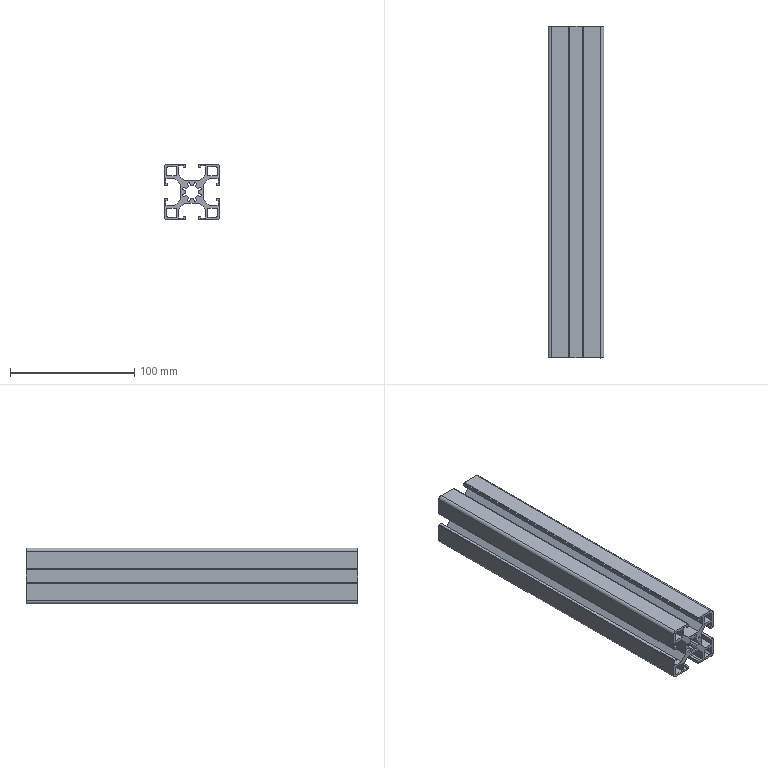Part | STEP file | 1 solid | 135 faces | box 45 x 267.5 x 45 mm | volume 185188 mm3 | plane 118 | cylinder 17 | commonest cylinder face diameters 10 x9 3 x4 5 x4